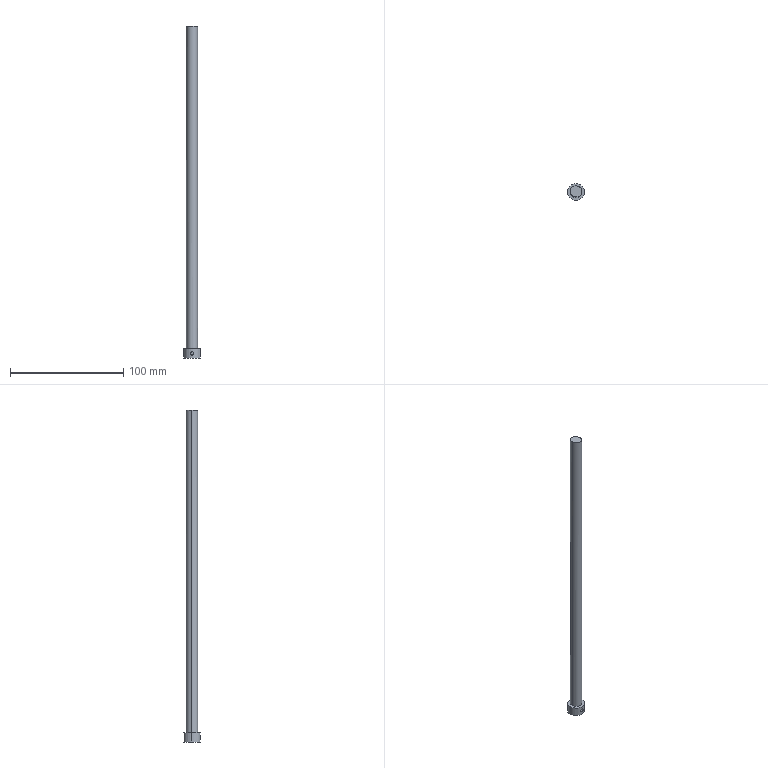Part | Creo | 1 solid | 10 faces | box 15 x 15 x 293.455 mm | volume 23765 mm3 | cylinder 6 | plane 4 | commonest cylinder face diameters 3 x2 10 x2 15 x2
STEP:
#1=CARTESIAN_POINT('',(66.,-141.,-252.5));
#2=VERTEX_POINT('',#1);
#3=CARTESIAN_POINT('',(56.,-141.,-252.5));
#4=VERTEX_POINT('',#3);
#5=CARTESIAN_POINT('',(61.,-141.,-252.5));
#6=DIRECTION('',(0.,0.,-1.));
#7=DIRECTION('',(1.,0.,0.));
#8=AXIS2_PLACEMENT_3D('',#5,#6,#7);
#9=CIRCLE('',#8,5.);
#10=EDGE_CURVE('',#2,#4,#9,.T.);
#11=ORIENTED_EDGE('',*,*,#10,.T.);
#12=CARTESIAN_POINT('',(56.,-141.,32.955));
#13=VERTEX_POINT('',#12);
#14=CARTESIAN_POINT('',(56.,-141.,32.955));
#15=DIRECTION('',(0.,0.,-1.));
#16=VECTOR('',#15,285.455);
#17=LINE('',#14,#16);
#18=EDGE_CURVE('',#13,#4,#17,.T.);
#19=ORIENTED_EDGE('',*,*,#18,.F.);
#20=CARTESIAN_POINT('',(66.,-141.,32.573));
#21=VERTEX_POINT('',#20);
#22=CARTESIAN_POINT('',(56.,-141.,32.955));
#23=CARTESIAN_POINT('',(56.,-141.589,32.955));
#24=CARTESIAN_POINT('',(56.215,-142.862,32.946));
#25=CARTESIAN_POINT('',(57.355,-144.641,32.903));
#26=CARTESIAN_POINT('',(59.15,-145.786,32.834));
#27=CARTESIAN_POINT('',(61.,-146.107,32.764));
#28=CARTESIAN_POINT('',(62.85,-145.786,32.693));
#29=CARTESIAN_POINT('',(64.645,-144.641,32.625));
#30=CARTESIAN_POINT('',(65.785,-142.862,32.581));
#31=CARTESIAN_POINT('',(66.,-141.589,32.573));
#32=CARTESIAN_POINT('',(66.,-141.,32.573));
#33=B_SPLINE_CURVE_WITH_KNOTS('',3,(#22,#23,#24,#25,#26,#27,#28,#29,#30,#31,#32),.UNSPECIFIED.,.F.,.F.,(4,1,1,1,1,1,1,1,4),(0.,0.125,0.25,0.375,0.5,0.625,0.75,0.875,1.),.UNSPECIFIED.);
#34=EDGE_CURVE('',#13,#21,#33,.T.);
#35=ORIENTED_EDGE('',*,*,#34,.T.);
#36=CARTESIAN_POINT('',(66.,-141.,32.573));
#37=DIRECTION('',(0.,0.,-1.));
#38=VECTOR('',#37,285.073);
#39=LINE('',#36,#38);
#40=EDGE_CURVE('',#21,#2,#39,.T.);
#41=ORIENTED_EDGE('',*,*,#40,.T.);
#42=EDGE_LOOP('',(#11,#19,#35,#41));
#43=FACE_OUTER_BOUND('',#42,.F.);
#44=CARTESIAN_POINT('',(61.,-141.,135.));
#45=DIRECTION('',(0.,0.,-1.));
#46=DIRECTION('',(1.,0.,0.));
#47=AXIS2_PLACEMENT_3D('',#44,#45,#46);
#48=CYLINDRICAL_SURFACE('',#47,5.);
#49=ADVANCED_FACE('',(#43),#48,.T.);
#50=CARTESIAN_POINT('',(53.5,-141.,-252.5));
#51=VERTEX_POINT('',#50);
#52=CARTESIAN_POINT('',(68.5,-141.,-252.5));
#53=VERTEX_POINT('',#52);
#54=CARTESIAN_POINT('',(61.,-141.,-252.5));
#55=DIRECTION('',(0.,0.,1.));
#56=DIRECTION('',(-1.,0.,0.));
#57=AXIS2_PLACEMENT_3D('',#54,#55,#56);
#58=CIRCLE('',#57,7.5);
#59=EDGE_CURVE('',#51,#53,#58,.T.);
#60=ORIENTED_EDGE('',*,*,#59,.F.);
#61=CARTESIAN_POINT('',(61.,-141.,-252.5));
#62=DIRECTION('',(0.,0.,1.));
#63=DIRECTION('',(1.,0.,0.));
#64=AXIS2_PLACEMENT_3D('',#61,#62,#63);
#65=CIRCLE('',#64,7.5);
#66=EDGE_CURVE('',#53,#51,#65,.T.);
#67=ORIENTED_EDGE('',*,*,#66,.F.);
#68=EDGE_LOOP('',(#60,#67));
#69=FACE_OUTER_BOUND('',#68,.F.);
#70=CARTESIAN_POINT('',(61.,-141.,-252.5));
#71=DIRECTION('',(0.,0.,-1.));
#72=DIRECTION('',(-1.,0.,0.));
#73=AXIS2_PLACEMENT_3D('',#70,#71,#72);
#74=CIRCLE('',#73,5.);
#75=EDGE_CURVE('',#4,#2,#74,.T.);
#76=ORIENTED_EDGE('',*,*,#75,.F.);
#77=ORIENTED_EDGE('',*,*,#10,.F.);
#78=EDGE_LOOP('',(#76,#77));
#79=FACE_BOUND('',#78,.F.);
#80=CARTESIAN_POINT('',(61.,-141.,-252.5));
#81=DIRECTION('',(0.,0.,1.));
#82=DIRECTION('',(-1.,0.,0.));
#83=AXIS2_PLACEMENT_3D('',#80,#81,#82);
#84=PLANE('',#83);
#85=ADVANCED_FACE('',(#69,#79),#84,.T.);
#86=ORIENTED_EDGE('',*,*,#75,.T.);
#87=ORIENTED_EDGE('',*,*,#40,.F.);
#88=CARTESIAN_POINT('',(66.,-141.,32.573));
#89=CARTESIAN_POINT('',(66.,-140.411,32.573));
#90=CARTESIAN_POINT('',(65.785,-139.138,32.581));
#91=CARTESIAN_POINT('',(64.645,-137.359,32.625));
#92=CARTESIAN_POINT('',(62.85,-136.214,32.693));
#93=CARTESIAN_POINT('',(61.,-135.893,32.764));
#94=CARTESIAN_POINT('',(59.15,-136.214,32.834));
#95=CARTESIAN_POINT('',(57.355,-137.359,32.903));
#96=CARTESIAN_POINT('',(56.215,-139.138,32.946));
#97=CARTESIAN_POINT('',(56.,-140.411,32.955));
#98=CARTESIAN_POINT('',(56.,-141.,32.955));
#99=B_SPLINE_CURVE_WITH_KNOTS('',3,(#88,#89,#90,#91,#92,#93,#94,#95,#96,#97,#98),.UNSPECIFIED.,.F.,.F.,(4,1,1,1,1,1,1,1,4),(0.,0.125,0.25,0.375,0.5,0.625,0.75,0.875,1.),.UNSPECIFIED.);
#100=EDGE_CURVE('',#21,#13,#99,.T.);
#101=ORIENTED_EDGE('',*,*,#100,.T.);
#102=ORIENTED_EDGE('',*,*,#18,.T.);
#103=EDGE_LOOP('',(#86,#87,#101,#102));
#104=FACE_OUTER_BOUND('',#103,.F.);
#105=CARTESIAN_POINT('',(61.,-141.,135.));
#106=DIRECTION('',(0.,0.,-1.));
#107=DIRECTION('',(1.,0.,0.));
#108=AXIS2_PLACEMENT_3D('',#105,#106,#107);
#109=CYLINDRICAL_SURFACE('',#108,5.);
#110=ADVANCED_FACE('',(#104),#109,.T.);
#111=ORIENTED_EDGE('',*,*,#100,.F.);
#112=ORIENTED_EDGE('',*,*,#34,.F.);
#113=EDGE_LOOP('',(#111,#112));
#114=FACE_OUTER_BOUND('',#113,.F.);
#115=CARTESIAN_POINT('',(0.9569,31.474,35.055));
#116=DIRECTION('',(0.03814,0.,0.9993));
#117=DIRECTION('',(0.9993,0.,-0.03814));
#118=AXIS2_PLACEMENT_3D('',#115,#116,#117);
#119=PLANE('',#118);
#120=ADVANCED_FACE('',(#114),#119,.T.);
#121=ORIENTED_EDGE('',*,*,#59,.T.);
#122=CARTESIAN_POINT('',(68.5,-141.,-260.5));
#123=VERTEX_POINT('',#122);
#124=CARTESIAN_POINT('',(68.5,-141.,-260.5));
#125=DIRECTION('',(0.,0.,1.));
#126=VECTOR('',#125,8.);
#127=LINE('',#124,#126);
#128=EDGE_CURVE('',#123,#53,#127,.T.);
#129=ORIENTED_EDGE('',*,*,#128,.F.);
#130=CARTESIAN_POINT('',(53.5,-141.,-260.5));
#131=VERTEX_POINT('',#130);
#132=CARTESIAN_POINT('',(61.,-141.,-260.5));
#133=DIRECTION('',(0.,0.,-1.));
#134=DIRECTION('',(1.,0.,0.));
#135=AXIS2_PLACEMENT_3D('',#132,#133,#134);
#136=CIRCLE('',#135,7.5);
#137=EDGE_CURVE('',#123,#131,#136,.T.);
#138=ORIENTED_EDGE('',*,*,#137,.T.);
#139=CARTESIAN_POINT('',(53.5,-141.,-260.5));
#140=DIRECTION('',(0.,0.,1.));
#141=VECTOR('',#140,8.);
#142=LINE('',#139,#141);
#143=EDGE_CURVE('',#131,#51,#142,.T.);
#144=ORIENTED_EDGE('',*,*,#143,.T.);
#145=EDGE_LOOP('',(#121,#129,#138,#144));
#146=FACE_OUTER_BOUND('',#145,.F.);
#147=CARTESIAN_POINT('',(61.,-148.5,-258.));
#148=VERTEX_POINT('',#147);
#149=CARTESIAN_POINT('',(61.,-148.5,-255.));
#150=VERTEX_POINT('',#149);
#151=CARTESIAN_POINT('',(61.,-148.5,-258.));
#152=CARTESIAN_POINT('',(60.795,-148.5,-258.));
#153=CARTESIAN_POINT('',(60.417,-148.484,-257.922));
#154=CARTESIAN_POINT('',(59.91,-148.425,-257.589));
#155=CARTESIAN_POINT('',(59.576,-148.365,-257.085));
#156=CARTESIAN_POINT('',(59.461,-148.34,-256.497));
#157=CARTESIAN_POINT('',(59.578,-148.365,-255.912));
#158=CARTESIAN_POINT('',(59.909,-148.425,-255.413));
#159=CARTESIAN_POINT('',(60.415,-148.484,-255.078));
#160=CARTESIAN_POINT('',(60.794,-148.5,-255.));
#161=CARTESIAN_POINT('',(61.,-148.5,-255.));
#162=B_SPLINE_CURVE_WITH_KNOTS('',3,(#151,#152,#153,#154,#155,#156,#157,#158,#159,#160,#161),.UNSPECIFIED.,.F.,.F.,(4,1,1,1,1,1,1,1,4),(0.,0.125,0.25,0.375,0.5,0.625,0.75,0.875,1.),.UNSPECIFIED.);
#163=EDGE_CURVE('',#148,#150,#162,.T.);
#164=ORIENTED_EDGE('',*,*,#163,.F.);
#165=CARTESIAN_POINT('',(61.,-148.5,-255.));
#166=CARTESIAN_POINT('',(61.206,-148.5,-255.));
#167=CARTESIAN_POINT('',(61.585,-148.484,-255.078));
#168=CARTESIAN_POINT('',(62.093,-148.424,-255.414));
#169=CARTESIAN_POINT('',(62.424,-148.364,-255.917));
#170=CARTESIAN_POINT('',(62.539,-148.34,-256.506));
#171=CARTESIAN_POINT('',(62.421,-148.365,-257.089));
#172=CARTESIAN_POINT('',(62.092,-148.424,-257.586));
#173=CARTESIAN_POINT('',(61.586,-148.484,-257.922));
#174=CARTESIAN_POINT('',(61.206,-148.5,-258.));
#175=CARTESIAN_POINT('',(61.,-148.5,-258.));
#176=B_SPLINE_CURVE_WITH_KNOTS('',3,(#165,#166,#167,#168,#169,#170,#171,#172,#173,#174,#175),.UNSPECIFIED.,.F.,.F.,(4,1,1,1,1,1,1,1,4),(0.,0.125,0.25,0.375,0.5,0.625,0.75,0.875,1.),.UNSPECIFIED.);
#177=EDGE_CURVE('',#150,#148,#176,.T.);
#178=ORIENTED_EDGE('',*,*,#177,.F.);
#179=EDGE_LOOP('',(#164,#178));
#180=FACE_BOUND('',#179,.F.);
#181=CARTESIAN_POINT('',(61.,-141.,-260.5));
#182=DIRECTION('',(0.,0.,1.));
#183=DIRECTION('',(-1.,0.,0.));
#184=AXIS2_PLACEMENT_3D('',#181,#182,#183);
#185=CYLINDRICAL_SURFACE('',#184,7.5);
#186=ADVANCED_FACE('',(#146,#180),#185,.T.);
#187=ORIENTED_EDGE('',*,*,#163,.T.);
#188=CARTESIAN_POINT('',(61.,-141.,-255.));
#189=VERTEX_POINT('',#188);
#190=CARTESIAN_POINT('',(61.,-141.,-255.));
#191=DIRECTION('',(0.000000004,-1.,-0.000006083));
#192=VECTOR('',#191,7.5);
#193=LINE('',#190,#192);
#194=EDGE_CURVE('',#189,#150,#193,.T.);
#195=ORIENTED_EDGE('',*,*,#194,.F.);
#196=CARTESIAN_POINT('',(61.,-141.,-258.));
#197=VERTEX_POINT('',#196);
#198=CARTESIAN_POINT('',(61.,-141.,-256.5));
#199=DIRECTION('',(0.,-1.,0.));
#200=DIRECTION('',(0.,0.,1.));
#201=AXIS2_PLACEMENT_3D('',#198,#199,#200);
#202=CIRCLE('',#201,1.5);
#203=EDGE_CURVE('',#189,#197,#202,.T.);
#204=ORIENTED_EDGE('',*,*,#203,.T.);
#205=CARTESIAN_POINT('',(61.,-141.,-258.));
#206=DIRECTION('',(0.,-1.,0.));
#207=VECTOR('',#206,7.5);
#208=LINE('',#205,#207);
#209=EDGE_CURVE('',#197,#148,#208,.T.);
#210=ORIENTED_EDGE('',*,*,#209,.T.);
#211=EDGE_LOOP('',(#187,#195,#204,#210));
#212=FACE_OUTER_BOUND('',#211,.F.);
#213=CARTESIAN_POINT('',(61.,-141.,-256.5));
#214=DIRECTION('',(0.,-1.,0.));
#215=DIRECTION('',(0.,0.,-1.));
#216=AXIS2_PLACEMENT_3D('',#213,#214,#215);
#217=CYLINDRICAL_SURFACE('',#216,1.5);
#218=ADVANCED_FACE('',(#212),#217,.F.);
#219=ORIENTED_EDGE('',*,*,#177,.T.);
#220=ORIENTED_EDGE('',*,*,#209,.F.);
#221=CARTESIAN_POINT('',(61.,-141.,-256.5));
#222=DIRECTION('',(0.,-1.,0.));
#223=DIRECTION('',(0.,0.,-1.));
#224=AXIS2_PLACEMENT_3D('',#221,#222,#223);
#225=CIRCLE('',#224,1.5);
#226=EDGE_CURVE('',#197,#189,#225,.T.);
#227=ORIENTED_EDGE('',*,*,#226,.T.);
#228=ORIENTED_EDGE('',*,*,#194,.T.);
#229=EDGE_LOOP('',(#219,#220,#227,#228));
#230=FACE_OUTER_BOUND('',#229,.F.);
#231=CARTESIAN_POINT('',(61.,-141.,-256.5));
#232=DIRECTION('',(0.,-1.,0.));
#233=DIRECTION('',(0.,0.,-1.));
#234=AXIS2_PLACEMENT_3D('',#231,#232,#233);
#235=CYLINDRICAL_SURFACE('',#234,1.5);
#236=ADVANCED_FACE('',(#230),#235,.F.);
#237=ORIENTED_EDGE('',*,*,#226,.F.);
#238=ORIENTED_EDGE('',*,*,#203,.F.);
#239=EDGE_LOOP('',(#237,#238));
#240=FACE_OUTER_BOUND('',#239,.F.);
#241=CARTESIAN_POINT('',(61.,-141.,-256.5));
#242=DIRECTION('',(0.,1.,0.));
#243=DIRECTION('',(0.,0.,1.));
#244=AXIS2_PLACEMENT_3D('',#241,#242,#243);
#245=PLANE('',#244);
#246=ADVANCED_FACE('',(#240),#245,.F.);
#247=ORIENTED_EDGE('',*,*,#66,.T.);
#248=ORIENTED_EDGE('',*,*,#143,.F.);
#249=CARTESIAN_POINT('',(61.,-141.,-260.5));
#250=DIRECTION('',(0.,0.,-1.));
#251=DIRECTION('',(-1.,0.,0.));
#252=AXIS2_PLACEMENT_3D('',#249,#250,#251);
#253=CIRCLE('',#252,7.5);
#254=EDGE_CURVE('',#131,#123,#253,.T.);
#255=ORIENTED_EDGE('',*,*,#254,.T.);
#256=ORIENTED_EDGE('',*,*,#128,.T.);
#257=EDGE_LOOP('',(#247,#248,#255,#256));
#258=FACE_OUTER_BOUND('',#257,.F.);
#259=CARTESIAN_POINT('',(61.,-141.,-260.5));
#260=DIRECTION('',(0.,0.,1.));
#261=DIRECTION('',(-1.,0.,0.));
#262=AXIS2_PLACEMENT_3D('',#259,#260,#261);
#263=CYLINDRICAL_SURFACE('',#262,7.5);
#264=ADVANCED_FACE('',(#258),#263,.T.);
#265=ORIENTED_EDGE('',*,*,#137,.F.);
#266=ORIENTED_EDGE('',*,*,#254,.F.);
#267=EDGE_LOOP('',(#265,#266));
#268=FACE_OUTER_BOUND('',#267,.F.);
#269=CARTESIAN_POINT('',(323.714,1.015,-260.5));
#270=DIRECTION('',(0.,0.,-1.));
#271=DIRECTION('',(1.,0.,0.));
#272=AXIS2_PLACEMENT_3D('',#269,#270,#271);
#273=PLANE('',#272);
#274=ADVANCED_FACE('',(#268),#273,.T.);
#275=CLOSED_SHELL('',(#49,#85,#110,#120,#186,#218,#236,#246,#264,#274));
#276=MANIFOLD_SOLID_BREP('',#275);
#277=(LENGTH_UNIT()NAMED_UNIT(*)SI_UNIT(.MILLI.,.METRE.));
#278=UNCERTAINTY_MEASURE_WITH_UNIT(LENGTH_MEASURE(0.02942),#277,'','');
#279=(NAMED_UNIT(*)PLANE_ANGLE_UNIT()SI_UNIT($,.RADIAN.));
#280=PLANE_ANGLE_MEASURE_WITH_UNIT(PLANE_ANGLE_MEASURE(0.01745),#279);
#281=(CONVERSION_BASED_UNIT('DEGREE',#280)NAMED_UNIT(*)PLANE_ANGLE_UNIT());
#282=(NAMED_UNIT(*)SI_UNIT($,.STERADIAN.)SOLID_ANGLE_UNIT());
#283=(GEOMETRIC_REPRESENTATION_CONTEXT(3)GLOBAL_UNCERTAINTY_ASSIGNED_CONTEXT((#278))GLOBAL_UNIT_ASSIGNED_CONTEXT((#277,#281,#282))REPRESENTATION_CONTEXT('',''));
#284=ADVANCED_BREP_SHAPE_REPRESENTATION('',(#276),#283);